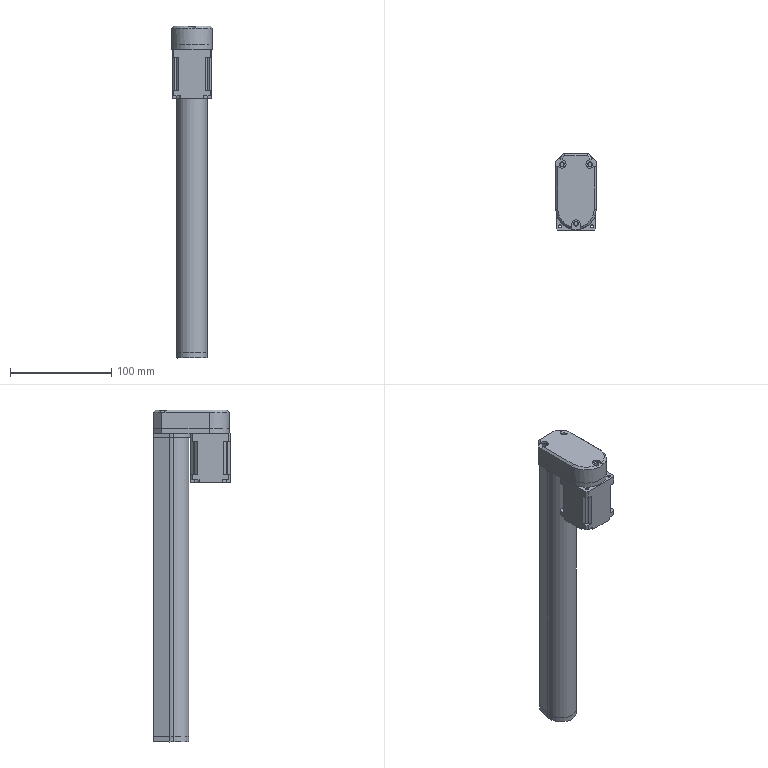Part | SolidWorks | features BaseBody 20 | 20 solids | 1774 faces | box 40 x 75.927 x 328 mm | volume 216478 mm3 | cylinder 1034 | spline 362 | plane 224 | torus 100 | sphere 48 | cone 6 | commonest cylinder face diameters 7.5 x251 10 x251 18 x70 15.75 x68 25 x57 22.75 x49